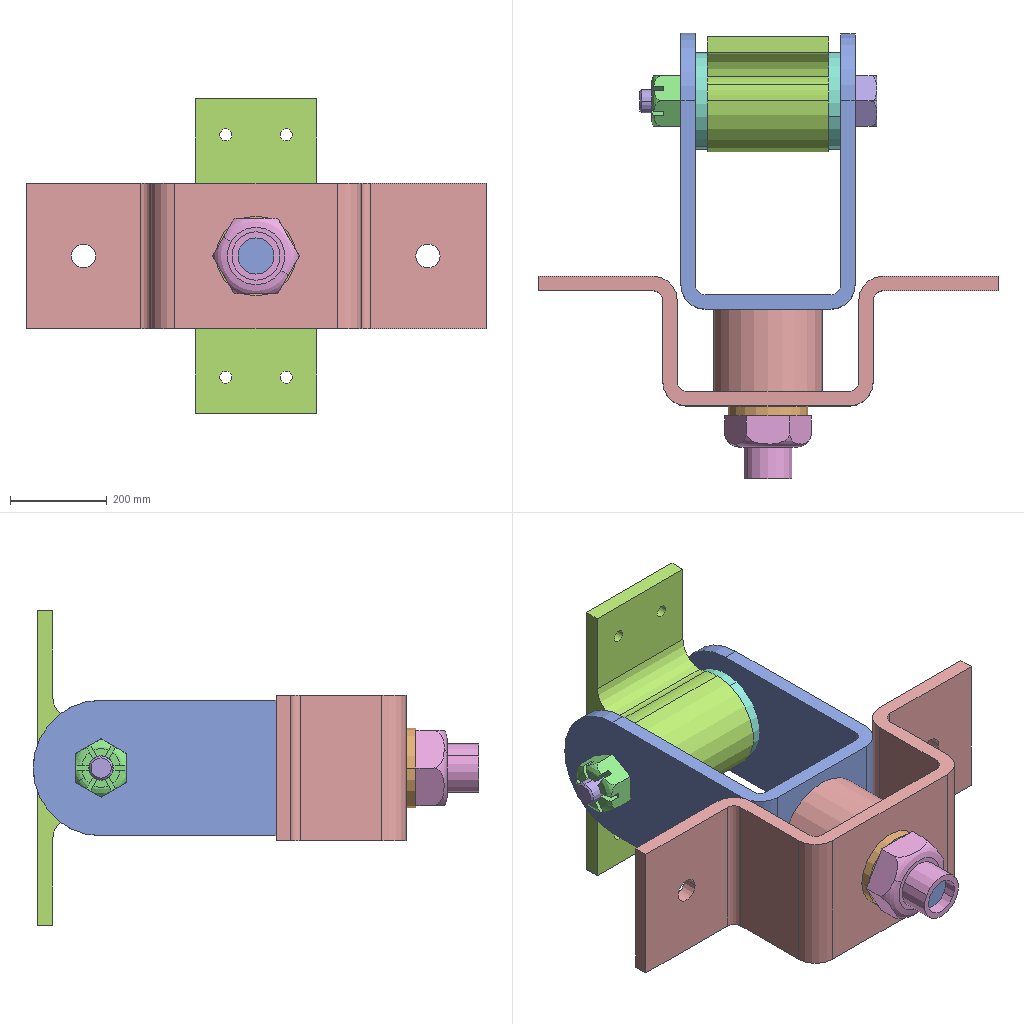Assembly | SolidWorks | 8 different items | 9 placed | box 950 x 920 x 650 mm
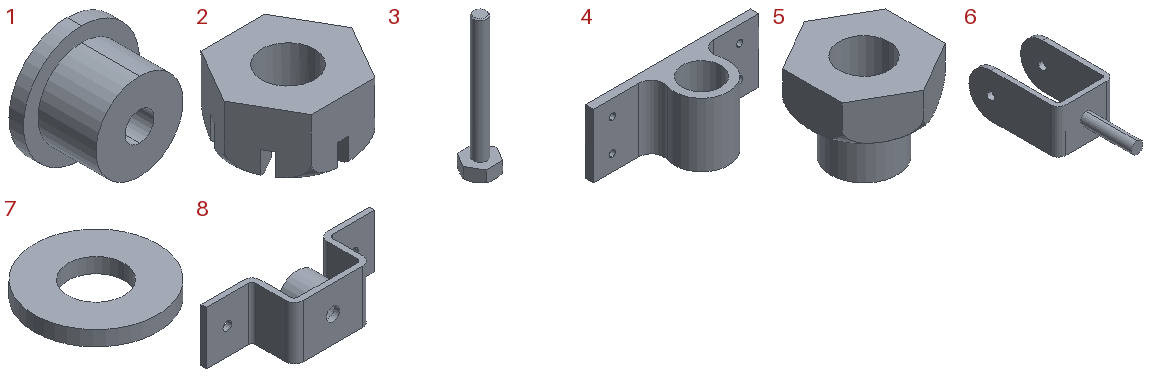Parts list (item | quantity | size | volume | features):
1 | x2 | 200 x 125 x 200 mm | 2307107 mm3 | features Revolution 1
2 | x1 | 120.089 x 104 x 60 mm | 394121 mm3 | features ICE 2, CirPattern 1, Extrusion 1, RevCut 1
3 | x1 | 120.089 x 104 x 490 mm | 1291940 mm3 | features Chamfer 1, Extrusion 1, ICE 1, RevCut 1
4 | x1 | 650 x 238 x 250 mm | 10403877 mm3 | features Extrusion 1, ICE 1
5 | x1 | 155 x 178.979 x 130 mm | 1254035 mm3 | features ICE 2, Extrusion 1, RevCut 1
6 | x1 | 360 x 895 x 280 mm | 12656881 mm3 | features ICE 6, Extrusion 1, Fillet 1
7 | x1 | 165 x 165 x 20 mm | 339292 mm3 | features Extrusion 1
8 | x1 | 950 x 268 x 300 mm | 14713211 mm3 | features Fillet 3, ICE 3, Extrusion 1
Mates (type | each side: item.copy, entity, surface, feature):
Coincident | 8.1 face plane Boss-Extrude3 | 6.1 face plane Boss-Extrude1
Parallel | 8.1 face plane Boss-Extrude2 | 6.1 face plane Boss-Extrude1
Concentric | 8.1 face cylinder Boss-Extrude3 | 6.1 face cylinder Boss-Extrude5
Concentric | 6.1 face cylinder Boss-Extrude5 | 7.1 face cylinder Boss-Extrude1
Coincident | 8.1 face plane Boss-Extrude2 | 7.1 face plane Boss-Extrude1
Coincident | 5.1 face plane Boss-Extrude1 | 7.1 face plane Boss-Extrude1
Concentric | 6.1 face cylinder Boss-Extrude5 | 5.1 face cylinder Boss-Extrude2
Parallel | 8.1 face plane Boss-Extrude2 | 5.1 face plane Boss-Extrude1
Coincident | 6.1 edge | 1.1 edge
Coincident | 6.1 edge | 1.2 edge
Concentric | 4.1 face cylinder Boss-Extrude1 | 1.2 face cylinder Revolve1
Parallel | 8.1 face plane Boss-Extrude2 | 4.1 face plane Boss-Extrude1
Coincident | 4.1 face plane Boss-Extrude1 | 1.2 face plane Revolve1
Concentric | 1.1 face cylinder Revolve1 | 3.1 face cylinder Boss-Extrude2
Coincident | 6.1 face plane Boss-Extrude1 | 3.1 face plane Boss-Extrude1
Concentric | 3.1 face cylinder Boss-Extrude2 | 2.1 face cylinder Cut-Extrude2
Coincident | 6.1 face plane Boss-Extrude1 | 2.1 face plane Boss-Extrude1
Parallel | 4.1 face plane Boss-Extrude1 | 2.1 face plane Boss-Extrude1
Parallel | 4.1 face plane Boss-Extrude1 | 3.1 face plane Boss-Extrude1